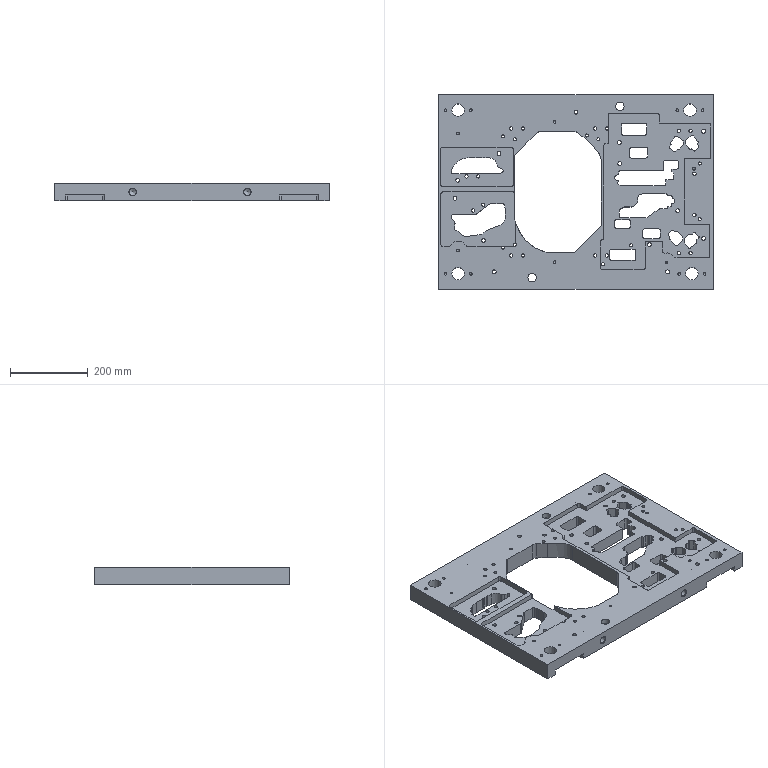Part | STEP file | 304_id158_x_t | 1 solid | 530 faces | box 705 x 500 x 45 mm | volume 9695540 mm3 | cylinder 241 | plane 158 | cone 76 | spline 55 | commonest cylinder face diameters 10 x66 8 x41 8.5 x37 6.8 x28 5.2 x8 7 x8